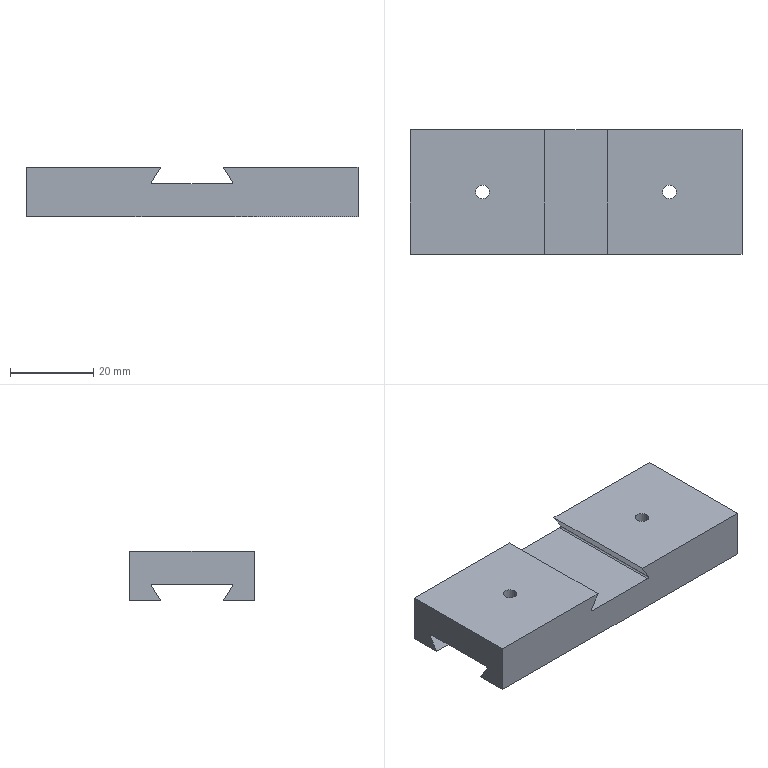Part | STEP file | slideway | 1 solid | 30 faces | box 80 x 30 x 12 mm | volume 20799 mm3 | plane 14 | cylinder 12 | cone 4 | commonest cylinder face diameters 3.3 x8 0.6 x4